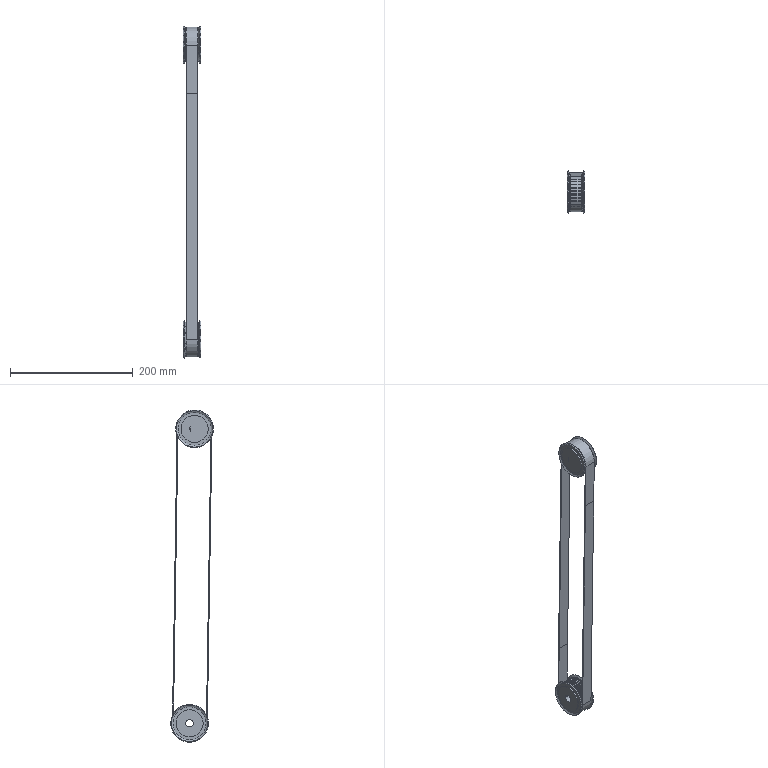Part | STEP file | _X2_51434EF6_X0_21_1 | 4 solids | 631 faces | box 29.173 x 69.582 x 540.649 mm | volume 150138 mm3 | cylinder 578 | plane 29 | cone 24 | commonest cylinder face diameters 1.075 x151 0.576 x142 7.584 x136 49.286 x63 53.549 x61 44.16 x8